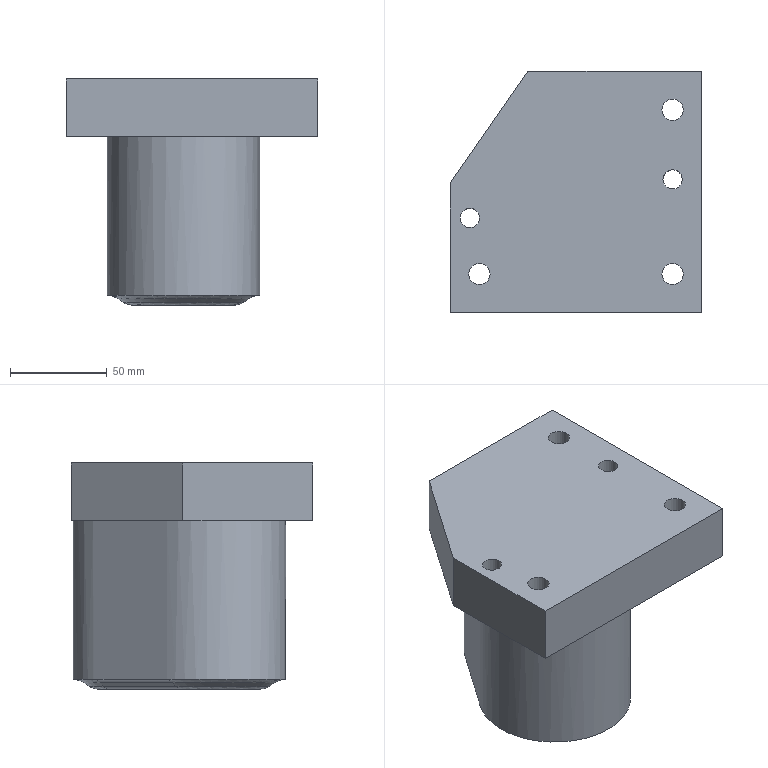Part | NX | features solid 2 | 1 solid | 32 faces | box 130 x 125 x 117 mm | volume 1001726 mm3 | spline 14 | plane 10 | cylinder 8 | commonest cylinder face diameters 11 x3 17.5 x3 10 x2